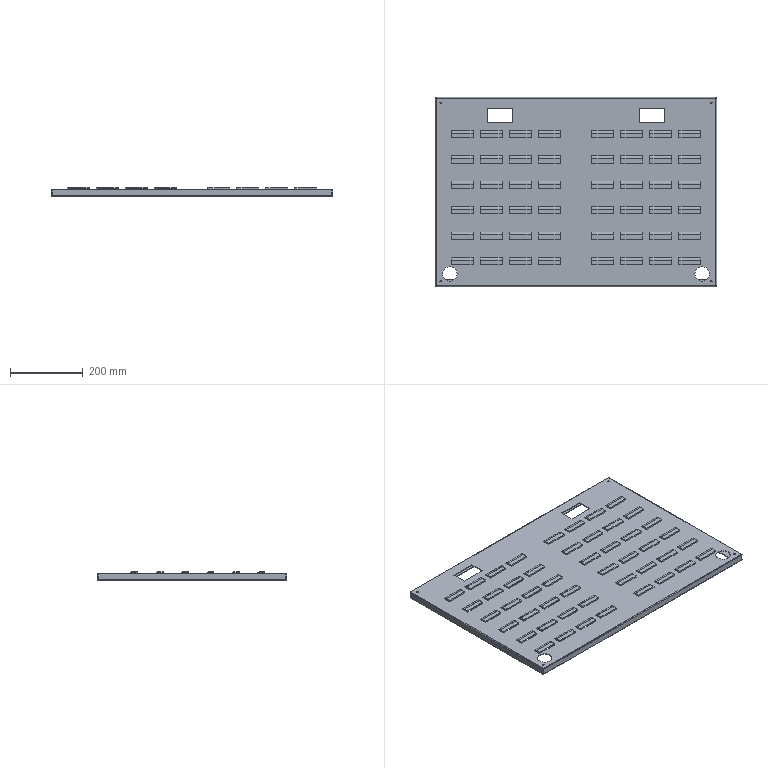Part | STEP file | 11-JX-00411 | 1 solid | 424 faces | box 775 x 521 x 24.03 mm | volume 1088417 mm3 | plane 312 | cylinder 104 | sphere 8 | commonest cylinder face diameters 16.441 x48 12.441 x24 4.5 x16 4 x12 40 x4